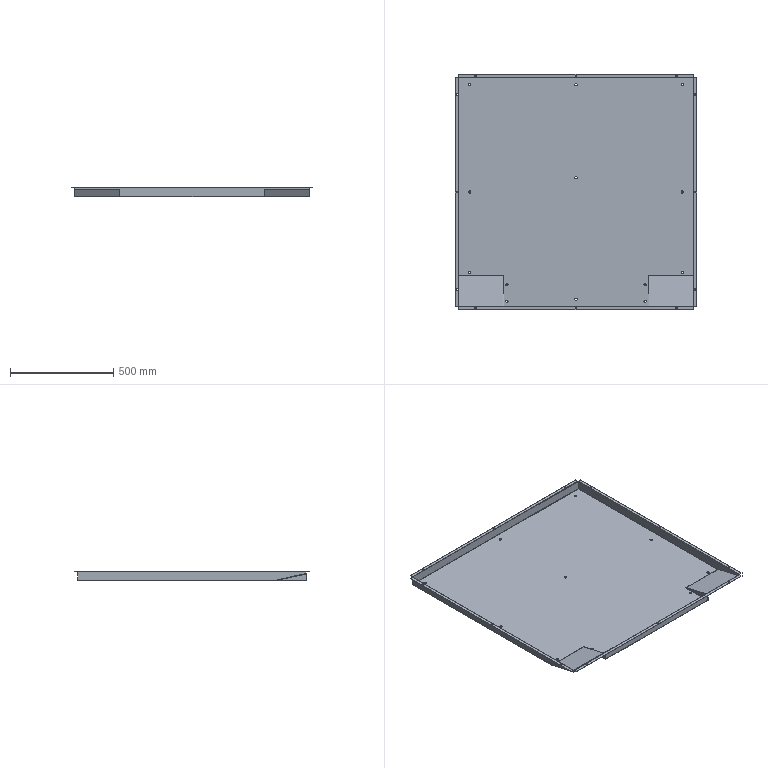Part | 3 solids | 186 faces | box 1170 x 1140 x 45 mm | volume 1511103 mm3 | plane 102 | cylinder 76 | spline 8 | commonest cylinder face diameters 7 x30 11 x26 0.4 x8 2.4 x8 2 x2 4 x2